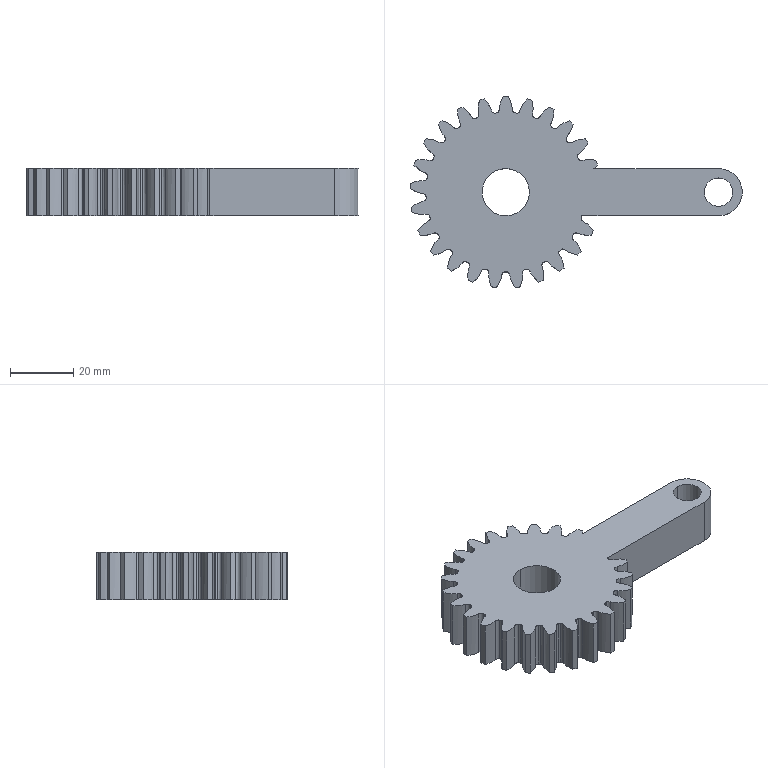Part | SolidWorks | features BaseBody 1 | 1 solid | 147 faces | box 105.355 x 60.601 x 15 mm | volume 43506 mm3 | spline 115 | cylinder 28 | plane 4 | commonest cylinder face diameters 50.625 x23 15 x3 9 x2